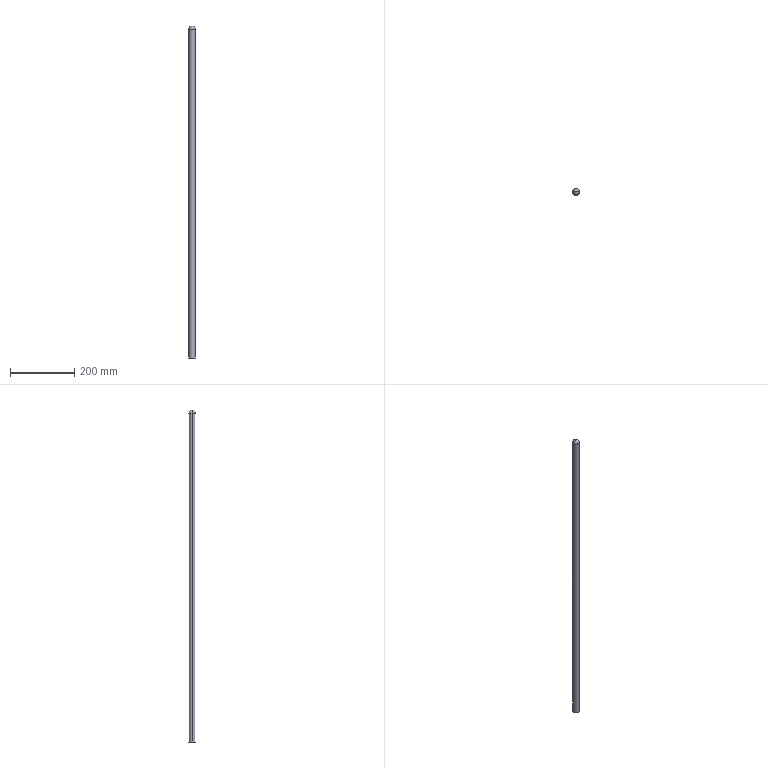Part | STEP file | X77-09003 | 1 solid | 6 faces | box 20 x 20 x 1030 mm | volume 322539 mm3 | torus 2 | cylinder 2 | plane 2 | commonest cylinder face diameters 20 x2
STEP:
#1=CARTESIAN_POINT('',(-10.,0.,1020.01));
#2=VERTEX_POINT('',#1);
#3=CARTESIAN_POINT('',(10.,0.,1020.01));
#4=VERTEX_POINT('',#3);
#5=CARTESIAN_POINT('',(0.,0.,1020.01));
#6=DIRECTION('',(0.,0.,-1.));
#7=DIRECTION('',(1.,0.,0.));
#8=AXIS2_PLACEMENT_3D('',#5,#6,#7);
#9=CIRCLE('',#8,10.);
#10=EDGE_CURVE('',#2,#4,#9,.T.);
#11=ORIENTED_EDGE('',*,*,#10,.F.);
#12=CARTESIAN_POINT('',(-0.01,0.,1030.));
#13=VERTEX_POINT('',#12);
#14=CARTESIAN_POINT('',(-0.01,0.,1020.01));
#15=DIRECTION('',(0.,1.,0.));
#16=DIRECTION('',(-1.,0.,0.));
#17=AXIS2_PLACEMENT_3D('',#14,#15,#16);
#18=CIRCLE('',#17,9.99);
#19=EDGE_CURVE('',#2,#13,#18,.T.);
#20=ORIENTED_EDGE('',*,*,#19,.T.);
#21=CARTESIAN_POINT('',(0.01,0.,1030.));
#22=VERTEX_POINT('',#21);
#23=CARTESIAN_POINT('',(0.,0.,1030.));
#24=DIRECTION('',(0.,0.,1.));
#25=DIRECTION('',(1.,0.,0.));
#26=AXIS2_PLACEMENT_3D('',#23,#24,#25);
#27=CIRCLE('',#26,0.01);
#28=EDGE_CURVE('',#22,#13,#27,.T.);
#29=ORIENTED_EDGE('',*,*,#28,.F.);
#30=CARTESIAN_POINT('',(0.01,0.,1020.01));
#31=DIRECTION('',(0.,-1.,0.));
#32=DIRECTION('',(0.,0.,-1.));
#33=AXIS2_PLACEMENT_3D('',#30,#31,#32);
#34=CIRCLE('',#33,9.99);
#35=EDGE_CURVE('',#4,#22,#34,.T.);
#36=ORIENTED_EDGE('',*,*,#35,.F.);
#37=EDGE_LOOP('',(#11,#20,#29,#36));
#38=FACE_OUTER_BOUND('',#37,.T.);
#39=CARTESIAN_POINT('',(0.,0.,1020.01));
#40=DIRECTION('',(0.,0.,1.));
#41=DIRECTION('',(1.,0.,0.));
#42=AXIS2_PLACEMENT_3D('',#39,#40,#41);
#43=TOROIDAL_SURFACE('',#42,0.01,9.99);
#44=ADVANCED_FACE('',(#38),#43,.T.);
#45=ORIENTED_EDGE('',*,*,#10,.T.);
#46=CARTESIAN_POINT('',(10.,0.,0.));
#47=VERTEX_POINT('',#46);
#48=CARTESIAN_POINT('',(10.,0.,1030.));
#49=DIRECTION('',(0.,0.,-1.));
#50=VECTOR('',#49,1000.);
#51=LINE('',#48,#50);
#52=EDGE_CURVE('',#4,#47,#51,.T.);
#53=ORIENTED_EDGE('',*,*,#52,.T.);
#54=CARTESIAN_POINT('',(-10.,0.,0.));
#55=VERTEX_POINT('',#54);
#56=CARTESIAN_POINT('',(0.,0.,0.));
#57=DIRECTION('',(0.,0.,1.));
#58=DIRECTION('',(1.,0.,0.));
#59=AXIS2_PLACEMENT_3D('',#56,#57,#58);
#60=CIRCLE('',#59,10.);
#61=EDGE_CURVE('',#47,#55,#60,.T.);
#62=ORIENTED_EDGE('',*,*,#61,.T.);
#63=CARTESIAN_POINT('',(-10.,0.,1030.));
#64=DIRECTION('',(0.,0.,-1.));
#65=VECTOR('',#64,1000.);
#66=LINE('',#63,#65);
#67=EDGE_CURVE('',#2,#55,#66,.T.);
#68=ORIENTED_EDGE('',*,*,#67,.F.);
#69=EDGE_LOOP('',(#45,#53,#62,#68));
#70=FACE_OUTER_BOUND('',#69,.T.);
#71=CARTESIAN_POINT('',(0.,0.,1030.));
#72=DIRECTION('',(0.,0.,-1.));
#73=DIRECTION('',(-1.,0.,0.));
#74=AXIS2_PLACEMENT_3D('',#71,#72,#73);
#75=CYLINDRICAL_SURFACE('',#74,10.);
#76=ADVANCED_FACE('',(#70),#75,.T.);
#77=ORIENTED_EDGE('',*,*,#52,.F.);
#78=CARTESIAN_POINT('',(0.,0.,1020.01));
#79=DIRECTION('',(0.,0.,-1.));
#80=DIRECTION('',(1.,0.,0.));
#81=AXIS2_PLACEMENT_3D('',#78,#79,#80);
#82=CIRCLE('',#81,10.);
#83=EDGE_CURVE('',#4,#2,#82,.T.);
#84=ORIENTED_EDGE('',*,*,#83,.T.);
#85=ORIENTED_EDGE('',*,*,#67,.T.);
#86=CARTESIAN_POINT('',(0.,0.,0.));
#87=DIRECTION('',(0.,0.,1.));
#88=DIRECTION('',(1.,0.,0.));
#89=AXIS2_PLACEMENT_3D('',#86,#87,#88);
#90=CIRCLE('',#89,10.);
#91=EDGE_CURVE('',#55,#47,#90,.T.);
#92=ORIENTED_EDGE('',*,*,#91,.T.);
#93=EDGE_LOOP('',(#77,#84,#85,#92));
#94=FACE_OUTER_BOUND('',#93,.T.);
#95=CARTESIAN_POINT('',(0.,0.,1030.));
#96=DIRECTION('',(0.,0.,-1.));
#97=DIRECTION('',(-1.,0.,0.));
#98=AXIS2_PLACEMENT_3D('',#95,#96,#97);
#99=CYLINDRICAL_SURFACE('',#98,10.);
#100=ADVANCED_FACE('',(#94),#99,.T.);
#101=ORIENTED_EDGE('',*,*,#28,.T.);
#102=CARTESIAN_POINT('',(0.,0.,1030.));
#103=DIRECTION('',(0.,0.,1.));
#104=DIRECTION('',(1.,0.,0.));
#105=AXIS2_PLACEMENT_3D('',#102,#103,#104);
#106=CIRCLE('',#105,0.01);
#107=EDGE_CURVE('',#13,#22,#106,.T.);
#108=ORIENTED_EDGE('',*,*,#107,.T.);
#109=EDGE_LOOP('',(#101,#108));
#110=FACE_OUTER_BOUND('',#109,.T.);
#111=CARTESIAN_POINT('',(0.,0.,1030.));
#112=DIRECTION('',(0.,0.,1.));
#113=DIRECTION('',(1.,0.,0.));
#114=AXIS2_PLACEMENT_3D('',#111,#112,#113);
#115=PLANE('',#114);
#116=ADVANCED_FACE('',(#110),#115,.T.);
#117=ORIENTED_EDGE('',*,*,#91,.F.);
#118=ORIENTED_EDGE('',*,*,#61,.F.);
#119=EDGE_LOOP('',(#117,#118));
#120=FACE_OUTER_BOUND('',#119,.T.);
#121=CARTESIAN_POINT('',(0.,0.,0.));
#122=DIRECTION('',(0.,0.,1.));
#123=DIRECTION('',(1.,0.,0.));
#124=AXIS2_PLACEMENT_3D('',#121,#122,#123);
#125=PLANE('',#124);
#126=ADVANCED_FACE('',(#120),#125,.F.);
#127=ORIENTED_EDGE('',*,*,#19,.F.);
#128=ORIENTED_EDGE('',*,*,#83,.F.);
#129=ORIENTED_EDGE('',*,*,#35,.T.);
#130=ORIENTED_EDGE('',*,*,#107,.F.);
#131=EDGE_LOOP('',(#127,#128,#129,#130));
#132=FACE_OUTER_BOUND('',#131,.T.);
#133=CARTESIAN_POINT('',(0.,0.,1020.01));
#134=DIRECTION('',(0.,0.,1.));
#135=DIRECTION('',(1.,0.,0.));
#136=AXIS2_PLACEMENT_3D('',#133,#134,#135);
#137=TOROIDAL_SURFACE('',#136,0.01,9.99);
#138=ADVANCED_FACE('',(#132),#137,.T.);
#139=CLOSED_SHELL('',(#44,#76,#100,#116,#126,#138));
#140=MANIFOLD_SOLID_BREP('',#139);
#141=CARTESIAN_POINT('',(0.,0.,0.));
#142=DIRECTION('',(0.,0.,1.));
#143=DIRECTION('',(1.,0.,0.));
#144=AXIS2_PLACEMENT_3D('',#141,#142,#143);
#145=(LENGTH_UNIT()NAMED_UNIT(*)SI_UNIT(.MILLI.,.METRE.));
#146=UNCERTAINTY_MEASURE_WITH_UNIT(LENGTH_MEASURE(0.00001),#145,'','');
#147=(NAMED_UNIT(*)PLANE_ANGLE_UNIT()SI_UNIT($,.RADIAN.));
#148=(NAMED_UNIT(*)SI_UNIT($,.STERADIAN.)SOLID_ANGLE_UNIT());
#149=(GEOMETRIC_REPRESENTATION_CONTEXT(3)GLOBAL_UNCERTAINTY_ASSIGNED_CONTEXT((#146))GLOBAL_UNIT_ASSIGNED_CONTEXT((#145,#147,#148))REPRESENTATION_CONTEXT('',''));
#150=ADVANCED_BREP_SHAPE_REPRESENTATION('',(#140,#144),#149);